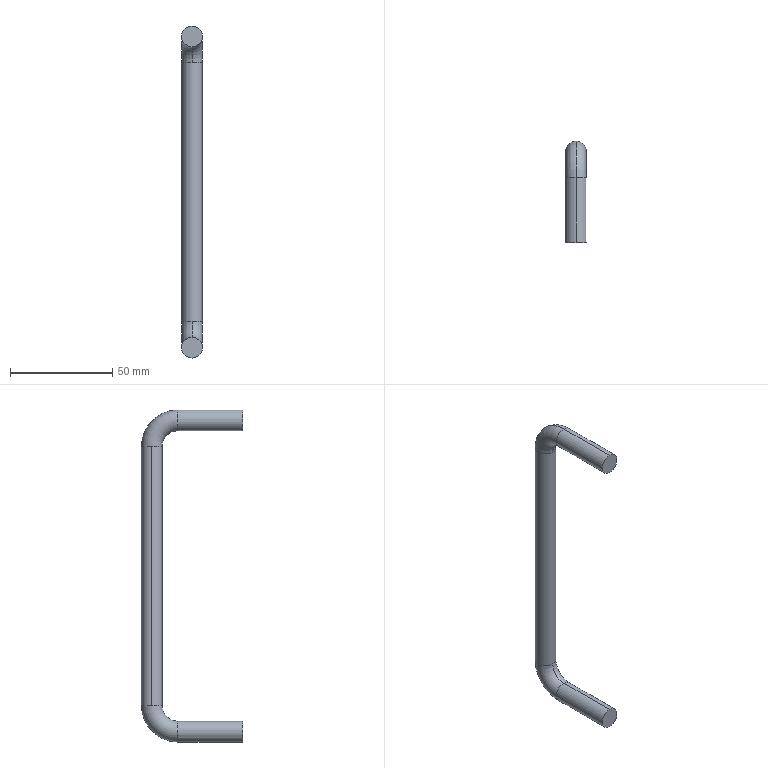Part | SolidWorks | features Sweep 1 | 1 solid | 12 faces | box 10.16 x 49.53 x 162.56 mm | volume 18679 mm3 | cylinder 6 | torus 4 | plane 2 | commonest cylinder face diameters 10.16 x6
STEP:
#1=CARTESIAN_POINT('',(0.,88.9,71.12));
#2=VERTEX_POINT('',#1);
#3=CARTESIAN_POINT('',(0.,88.9,81.28));
#4=VERTEX_POINT('',#3);
#5=CARTESIAN_POINT('',(0.,88.9,76.2));
#6=DIRECTION('',(0.,1.,0.));
#7=DIRECTION('',(0.,0.,1.));
#8=AXIS2_PLACEMENT_3D('',#5,#6,#7);
#9=CIRCLE('',#8,5.08);
#10=EDGE_CURVE('',#2,#4,#9,.T.);
#11=ORIENTED_EDGE('',*,*,#10,.T.);
#12=CARTESIAN_POINT('',(0.,106.68,63.5));
#13=VERTEX_POINT('',#12);
#14=CARTESIAN_POINT('',(0.,88.9,63.5));
#15=DIRECTION('',(-1.,0.,0.));
#16=DIRECTION('',(0.,0.,1.));
#17=AXIS2_PLACEMENT_3D('',#14,#15,#16);
#18=CIRCLE('',#17,17.78);
#19=EDGE_CURVE('',#4,#13,#18,.T.);
#20=ORIENTED_EDGE('',*,*,#19,.T.);
#21=CARTESIAN_POINT('',(-5.08,101.6,63.5));
#22=VERTEX_POINT('',#21);
#23=CARTESIAN_POINT('',(0.,101.6,63.5));
#24=DIRECTION('',(0.,0.,-1.));
#25=DIRECTION('',(0.,1.,0.));
#26=AXIS2_PLACEMENT_3D('',#23,#24,#25);
#27=CIRCLE('',#26,5.08);
#28=EDGE_CURVE('',#22,#13,#27,.T.);
#29=ORIENTED_EDGE('',*,*,#28,.F.);
#30=CARTESIAN_POINT('',(0.,96.52,63.5));
#31=VERTEX_POINT('',#30);
#32=CARTESIAN_POINT('',(0.,101.6,63.5));
#33=DIRECTION('',(0.,0.,-1.));
#34=DIRECTION('',(0.,1.,0.));
#35=AXIS2_PLACEMENT_3D('',#32,#33,#34);
#36=CIRCLE('',#35,5.08);
#37=EDGE_CURVE('',#31,#22,#36,.T.);
#38=ORIENTED_EDGE('',*,*,#37,.F.);
#39=CARTESIAN_POINT('',(0.,88.9,63.5));
#40=DIRECTION('',(-1.,0.,0.));
#41=DIRECTION('',(0.,0.,1.));
#42=AXIS2_PLACEMENT_3D('',#39,#40,#41);
#43=CIRCLE('',#42,7.62);
#44=EDGE_CURVE('',#2,#31,#43,.T.);
#45=ORIENTED_EDGE('',*,*,#44,.F.);
#46=EDGE_LOOP('',(#11,#20,#29,#38,#45));
#47=FACE_OUTER_BOUND('',#46,.T.);
#48=CARTESIAN_POINT('',(0.,88.9,63.5));
#49=DIRECTION('',(-1.,0.,0.));
#50=DIRECTION('',(0.,0.,1.));
#51=AXIS2_PLACEMENT_3D('',#48,#49,#50);
#52=TOROIDAL_SURFACE('',#51,12.7,5.08);
#53=ADVANCED_FACE('',(#47),#52,.T.);
#54=CARTESIAN_POINT('',(-5.08,101.6,-63.5));
#55=VERTEX_POINT('',#54);
#56=CARTESIAN_POINT('',(0.,106.68,-63.5));
#57=VERTEX_POINT('',#56);
#58=CARTESIAN_POINT('',(0.,101.6,-63.5));
#59=DIRECTION('',(0.,0.,-1.));
#60=DIRECTION('',(0.,1.,0.));
#61=AXIS2_PLACEMENT_3D('',#58,#59,#60);
#62=CIRCLE('',#61,5.08);
#63=EDGE_CURVE('',#55,#57,#62,.T.);
#64=ORIENTED_EDGE('',*,*,#63,.T.);
#65=CARTESIAN_POINT('',(0.,88.9,-81.28));
#66=VERTEX_POINT('',#65);
#67=CARTESIAN_POINT('',(0.,88.9,-63.5));
#68=DIRECTION('',(-1.,0.,0.));
#69=DIRECTION('',(0.,0.,1.));
#70=AXIS2_PLACEMENT_3D('',#67,#68,#69);
#71=CIRCLE('',#70,17.78);
#72=EDGE_CURVE('',#57,#66,#71,.T.);
#73=ORIENTED_EDGE('',*,*,#72,.T.);
#74=CARTESIAN_POINT('',(0.,88.9,-71.12));
#75=VERTEX_POINT('',#74);
#76=CARTESIAN_POINT('',(0.,88.9,-76.2));
#77=DIRECTION('',(0.,-1.,0.));
#78=DIRECTION('',(0.,0.,-1.));
#79=AXIS2_PLACEMENT_3D('',#76,#77,#78);
#80=CIRCLE('',#79,5.08);
#81=EDGE_CURVE('',#75,#66,#80,.T.);
#82=ORIENTED_EDGE('',*,*,#81,.F.);
#83=CARTESIAN_POINT('',(0.,96.52,-63.5));
#84=VERTEX_POINT('',#83);
#85=CARTESIAN_POINT('',(0.,88.9,-63.5));
#86=DIRECTION('',(-1.,0.,0.));
#87=DIRECTION('',(0.,0.,1.));
#88=AXIS2_PLACEMENT_3D('',#85,#86,#87);
#89=CIRCLE('',#88,7.62);
#90=EDGE_CURVE('',#84,#75,#89,.T.);
#91=ORIENTED_EDGE('',*,*,#90,.F.);
#92=CARTESIAN_POINT('',(0.,101.6,-63.5));
#93=DIRECTION('',(0.,0.,-1.));
#94=DIRECTION('',(0.,1.,0.));
#95=AXIS2_PLACEMENT_3D('',#92,#93,#94);
#96=CIRCLE('',#95,5.08);
#97=EDGE_CURVE('',#84,#55,#96,.T.);
#98=ORIENTED_EDGE('',*,*,#97,.T.);
#99=EDGE_LOOP('',(#64,#73,#82,#91,#98));
#100=FACE_OUTER_BOUND('',#99,.T.);
#101=CARTESIAN_POINT('',(0.,88.9,-63.5));
#102=DIRECTION('',(-1.,0.,0.));
#103=DIRECTION('',(0.,0.,1.));
#104=AXIS2_PLACEMENT_3D('',#101,#102,#103);
#105=TOROIDAL_SURFACE('',#104,12.7,5.08);
#106=ADVANCED_FACE('',(#100),#105,.T.);
#107=CARTESIAN_POINT('',(0.,88.9,76.2));
#108=DIRECTION('',(0.,1.,0.));
#109=DIRECTION('',(0.,0.,1.));
#110=AXIS2_PLACEMENT_3D('',#107,#108,#109);
#111=CIRCLE('',#110,5.08);
#112=EDGE_CURVE('',#4,#2,#111,.T.);
#113=ORIENTED_EDGE('',*,*,#112,.F.);
#114=CARTESIAN_POINT('',(0.,57.15,81.28));
#115=VERTEX_POINT('',#114);
#116=CARTESIAN_POINT('',(0.,88.9,81.28));
#117=DIRECTION('',(0.,-1.,0.));
#118=VECTOR('',#117,1000.);
#119=LINE('',#116,#118);
#120=EDGE_CURVE('',#4,#115,#119,.T.);
#121=ORIENTED_EDGE('',*,*,#120,.T.);
#122=CARTESIAN_POINT('',(0.,57.15,71.12));
#123=VERTEX_POINT('',#122);
#124=CARTESIAN_POINT('',(0.,57.15,76.2));
#125=DIRECTION('',(0.,1.,0.));
#126=DIRECTION('',(0.,0.,1.));
#127=AXIS2_PLACEMENT_3D('',#124,#125,#126);
#128=CIRCLE('',#127,5.08);
#129=EDGE_CURVE('',#115,#123,#128,.T.);
#130=ORIENTED_EDGE('',*,*,#129,.T.);
#131=CARTESIAN_POINT('',(0.,88.9,71.12));
#132=DIRECTION('',(0.,-1.,0.));
#133=VECTOR('',#132,1000.);
#134=LINE('',#131,#133);
#135=EDGE_CURVE('',#2,#123,#134,.T.);
#136=ORIENTED_EDGE('',*,*,#135,.F.);
#137=EDGE_LOOP('',(#113,#121,#130,#136));
#138=FACE_OUTER_BOUND('',#137,.T.);
#139=CARTESIAN_POINT('',(0.,88.9,76.2));
#140=DIRECTION('',(0.,-1.,0.));
#141=DIRECTION('',(0.,0.,-1.));
#142=AXIS2_PLACEMENT_3D('',#139,#140,#141);
#143=CYLINDRICAL_SURFACE('',#142,5.08);
#144=ADVANCED_FACE('',(#138),#143,.T.);
#145=ORIENTED_EDGE('',*,*,#28,.T.);
#146=CARTESIAN_POINT('',(5.08,101.6,63.5));
#147=VERTEX_POINT('',#146);
#148=CARTESIAN_POINT('',(0.,101.6,63.5));
#149=DIRECTION('',(0.,0.,-1.));
#150=DIRECTION('',(0.,1.,0.));
#151=AXIS2_PLACEMENT_3D('',#148,#149,#150);
#152=CIRCLE('',#151,5.08);
#153=EDGE_CURVE('',#13,#147,#152,.T.);
#154=ORIENTED_EDGE('',*,*,#153,.T.);
#155=CARTESIAN_POINT('',(5.08,101.6,-63.5));
#156=VERTEX_POINT('',#155);
#157=CARTESIAN_POINT('',(5.08,101.6,63.5));
#158=DIRECTION('',(0.,0.,-1.));
#159=VECTOR('',#158,1000.);
#160=LINE('',#157,#159);
#161=EDGE_CURVE('',#147,#156,#160,.T.);
#162=ORIENTED_EDGE('',*,*,#161,.T.);
#163=CARTESIAN_POINT('',(0.,101.6,-63.5));
#164=DIRECTION('',(0.,0.,-1.));
#165=DIRECTION('',(0.,1.,0.));
#166=AXIS2_PLACEMENT_3D('',#163,#164,#165);
#167=CIRCLE('',#166,5.08);
#168=EDGE_CURVE('',#57,#156,#167,.T.);
#169=ORIENTED_EDGE('',*,*,#168,.F.);
#170=ORIENTED_EDGE('',*,*,#63,.F.);
#171=CARTESIAN_POINT('',(-5.08,101.6,63.5));
#172=DIRECTION('',(0.,0.,-1.));
#173=VECTOR('',#172,1000.);
#174=LINE('',#171,#173);
#175=EDGE_CURVE('',#22,#55,#174,.T.);
#176=ORIENTED_EDGE('',*,*,#175,.F.);
#177=EDGE_LOOP('',(#145,#154,#162,#169,#170,#176));
#178=FACE_OUTER_BOUND('',#177,.T.);
#179=CARTESIAN_POINT('',(0.,101.6,63.5));
#180=DIRECTION('',(0.,0.,-1.));
#181=DIRECTION('',(-1.,0.,0.));
#182=AXIS2_PLACEMENT_3D('',#179,#180,#181);
#183=CYLINDRICAL_SURFACE('',#182,5.08);
#184=ADVANCED_FACE('',(#178),#183,.T.);
#185=CARTESIAN_POINT('',(0.,88.9,-76.2));
#186=DIRECTION('',(0.,-1.,0.));
#187=DIRECTION('',(0.,0.,-1.));
#188=AXIS2_PLACEMENT_3D('',#185,#186,#187);
#189=CIRCLE('',#188,5.08);
#190=EDGE_CURVE('',#66,#75,#189,.T.);
#191=ORIENTED_EDGE('',*,*,#190,.T.);
#192=CARTESIAN_POINT('',(0.,57.15,-71.12));
#193=VERTEX_POINT('',#192);
#194=CARTESIAN_POINT('',(0.,88.9,-71.12));
#195=DIRECTION('',(0.,-1.,0.));
#196=VECTOR('',#195,1000.);
#197=LINE('',#194,#196);
#198=EDGE_CURVE('',#75,#193,#197,.T.);
#199=ORIENTED_EDGE('',*,*,#198,.T.);
#200=CARTESIAN_POINT('',(0.,57.15,-81.28));
#201=VERTEX_POINT('',#200);
#202=CARTESIAN_POINT('',(0.,57.15,-76.2));
#203=DIRECTION('',(0.,-1.,0.));
#204=DIRECTION('',(0.,0.,-1.));
#205=AXIS2_PLACEMENT_3D('',#202,#203,#204);
#206=CIRCLE('',#205,5.08);
#207=EDGE_CURVE('',#201,#193,#206,.T.);
#208=ORIENTED_EDGE('',*,*,#207,.F.);
#209=CARTESIAN_POINT('',(0.,88.9,-81.28));
#210=DIRECTION('',(0.,-1.,0.));
#211=VECTOR('',#210,1000.);
#212=LINE('',#209,#211);
#213=EDGE_CURVE('',#66,#201,#212,.T.);
#214=ORIENTED_EDGE('',*,*,#213,.F.);
#215=EDGE_LOOP('',(#191,#199,#208,#214));
#216=FACE_OUTER_BOUND('',#215,.T.);
#217=CARTESIAN_POINT('',(0.,88.9,-76.2));
#218=DIRECTION('',(0.,-1.,0.));
#219=DIRECTION('',(0.,0.,-1.));
#220=AXIS2_PLACEMENT_3D('',#217,#218,#219);
#221=CYLINDRICAL_SURFACE('',#220,5.08);
#222=ADVANCED_FACE('',(#216),#221,.T.);
#223=ORIENTED_EDGE('',*,*,#198,.F.);
#224=ORIENTED_EDGE('',*,*,#81,.T.);
#225=ORIENTED_EDGE('',*,*,#213,.T.);
#226=CARTESIAN_POINT('',(0.,57.15,-76.2));
#227=DIRECTION('',(0.,-1.,0.));
#228=DIRECTION('',(0.,0.,-1.));
#229=AXIS2_PLACEMENT_3D('',#226,#227,#228);
#230=CIRCLE('',#229,5.08);
#231=EDGE_CURVE('',#193,#201,#230,.T.);
#232=ORIENTED_EDGE('',*,*,#231,.F.);
#233=EDGE_LOOP('',(#223,#224,#225,#232));
#234=FACE_OUTER_BOUND('',#233,.T.);
#235=CARTESIAN_POINT('',(0.,88.9,-76.2));
#236=DIRECTION('',(0.,-1.,0.));
#237=DIRECTION('',(0.,0.,-1.));
#238=AXIS2_PLACEMENT_3D('',#235,#236,#237);
#239=CYLINDRICAL_SURFACE('',#238,5.08);
#240=ADVANCED_FACE('',(#234),#239,.T.);
#241=ORIENTED_EDGE('',*,*,#72,.F.);
#242=ORIENTED_EDGE('',*,*,#168,.T.);
#243=CARTESIAN_POINT('',(0.,101.6,-63.5));
#244=DIRECTION('',(0.,0.,-1.));
#245=DIRECTION('',(0.,1.,0.));
#246=AXIS2_PLACEMENT_3D('',#243,#244,#245);
#247=CIRCLE('',#246,5.08);
#248=EDGE_CURVE('',#156,#84,#247,.T.);
#249=ORIENTED_EDGE('',*,*,#248,.T.);
#250=ORIENTED_EDGE('',*,*,#90,.T.);
#251=ORIENTED_EDGE('',*,*,#190,.F.);
#252=EDGE_LOOP('',(#241,#242,#249,#250,#251));
#253=FACE_OUTER_BOUND('',#252,.T.);
#254=CARTESIAN_POINT('',(0.,88.9,-63.5));
#255=DIRECTION('',(-1.,0.,0.));
#256=DIRECTION('',(0.,0.,1.));
#257=AXIS2_PLACEMENT_3D('',#254,#255,#256);
#258=TOROIDAL_SURFACE('',#257,12.7,5.08);
#259=ADVANCED_FACE('',(#253),#258,.T.);
#260=ORIENTED_EDGE('',*,*,#161,.F.);
#261=CARTESIAN_POINT('',(0.,101.6,63.5));
#262=DIRECTION('',(0.,0.,-1.));
#263=DIRECTION('',(0.,1.,0.));
#264=AXIS2_PLACEMENT_3D('',#261,#262,#263);
#265=CIRCLE('',#264,5.08);
#266=EDGE_CURVE('',#147,#31,#265,.T.);
#267=ORIENTED_EDGE('',*,*,#266,.T.);
#268=ORIENTED_EDGE('',*,*,#37,.T.);
#269=ORIENTED_EDGE('',*,*,#175,.T.);
#270=ORIENTED_EDGE('',*,*,#97,.F.);
#271=ORIENTED_EDGE('',*,*,#248,.F.);
#272=EDGE_LOOP('',(#260,#267,#268,#269,#270,#271));
#273=FACE_OUTER_BOUND('',#272,.T.);
#274=CARTESIAN_POINT('',(0.,101.6,63.5));
#275=DIRECTION('',(0.,0.,-1.));
#276=DIRECTION('',(-1.,0.,0.));
#277=AXIS2_PLACEMENT_3D('',#274,#275,#276);
#278=CYLINDRICAL_SURFACE('',#277,5.08);
#279=ADVANCED_FACE('',(#273),#278,.T.);
#280=ORIENTED_EDGE('',*,*,#19,.F.);
#281=ORIENTED_EDGE('',*,*,#112,.T.);
#282=ORIENTED_EDGE('',*,*,#44,.T.);
#283=ORIENTED_EDGE('',*,*,#266,.F.);
#284=ORIENTED_EDGE('',*,*,#153,.F.);
#285=EDGE_LOOP('',(#280,#281,#282,#283,#284));
#286=FACE_OUTER_BOUND('',#285,.T.);
#287=CARTESIAN_POINT('',(0.,88.9,63.5));
#288=DIRECTION('',(-1.,0.,0.));
#289=DIRECTION('',(0.,0.,1.));
#290=AXIS2_PLACEMENT_3D('',#287,#288,#289);
#291=TOROIDAL_SURFACE('',#290,12.7,5.08);
#292=ADVANCED_FACE('',(#286),#291,.T.);
#293=ORIENTED_EDGE('',*,*,#120,.F.);
#294=ORIENTED_EDGE('',*,*,#10,.F.);
#295=ORIENTED_EDGE('',*,*,#135,.T.);
#296=CARTESIAN_POINT('',(0.,57.15,76.2));
#297=DIRECTION('',(0.,1.,0.));
#298=DIRECTION('',(0.,0.,1.));
#299=AXIS2_PLACEMENT_3D('',#296,#297,#298);
#300=CIRCLE('',#299,5.08);
#301=EDGE_CURVE('',#123,#115,#300,.T.);
#302=ORIENTED_EDGE('',*,*,#301,.T.);
#303=EDGE_LOOP('',(#293,#294,#295,#302));
#304=FACE_OUTER_BOUND('',#303,.T.);
#305=CARTESIAN_POINT('',(0.,88.9,76.2));
#306=DIRECTION('',(0.,-1.,0.));
#307=DIRECTION('',(0.,0.,-1.));
#308=AXIS2_PLACEMENT_3D('',#305,#306,#307);
#309=CYLINDRICAL_SURFACE('',#308,5.08);
#310=ADVANCED_FACE('',(#304),#309,.T.);
#311=ORIENTED_EDGE('',*,*,#207,.T.);
#312=ORIENTED_EDGE('',*,*,#231,.T.);
#313=EDGE_LOOP('',(#311,#312));
#314=FACE_OUTER_BOUND('',#313,.T.);
#315=CARTESIAN_POINT('',(0.,57.15,-76.2));
#316=DIRECTION('',(0.,-1.,0.));
#317=DIRECTION('',(0.,0.,-1.));
#318=AXIS2_PLACEMENT_3D('',#315,#316,#317);
#319=PLANE('',#318);
#320=ADVANCED_FACE('',(#314),#319,.T.);
#321=ORIENTED_EDGE('',*,*,#301,.F.);
#322=ORIENTED_EDGE('',*,*,#129,.F.);
#323=EDGE_LOOP('',(#321,#322));
#324=FACE_OUTER_BOUND('',#323,.T.);
#325=CARTESIAN_POINT('',(0.,57.15,76.2));
#326=DIRECTION('',(0.,1.,0.));
#327=DIRECTION('',(0.,0.,1.));
#328=AXIS2_PLACEMENT_3D('',#325,#326,#327);
#329=PLANE('',#328);
#330=ADVANCED_FACE('',(#324),#329,.F.);
#331=CLOSED_SHELL('',(#53,#106,#144,#184,#222,#240,#259,#279,#292,#310,#320,#330));
#332=MANIFOLD_SOLID_BREP('',#331);
#333=CARTESIAN_POINT('',(0.,0.,0.));
#334=DIRECTION('',(0.,0.,1.));
#335=DIRECTION('',(1.,0.,0.));
#336=AXIS2_PLACEMENT_3D('',#333,#334,#335);
#337=(LENGTH_UNIT()NAMED_UNIT(*)SI_UNIT(.MILLI.,.METRE.));
#338=UNCERTAINTY_MEASURE_WITH_UNIT(LENGTH_MEASURE(0.00001),#337,'','');
#339=(NAMED_UNIT(*)PLANE_ANGLE_UNIT()SI_UNIT($,.RADIAN.));
#340=(NAMED_UNIT(*)SI_UNIT($,.STERADIAN.)SOLID_ANGLE_UNIT());
#341=(GEOMETRIC_REPRESENTATION_CONTEXT(3)GLOBAL_UNCERTAINTY_ASSIGNED_CONTEXT((#338))GLOBAL_UNIT_ASSIGNED_CONTEXT((#337,#339,#340))REPRESENTATION_CONTEXT('',''));
#342=ADVANCED_BREP_SHAPE_REPRESENTATION('',(#332,#336),#341);